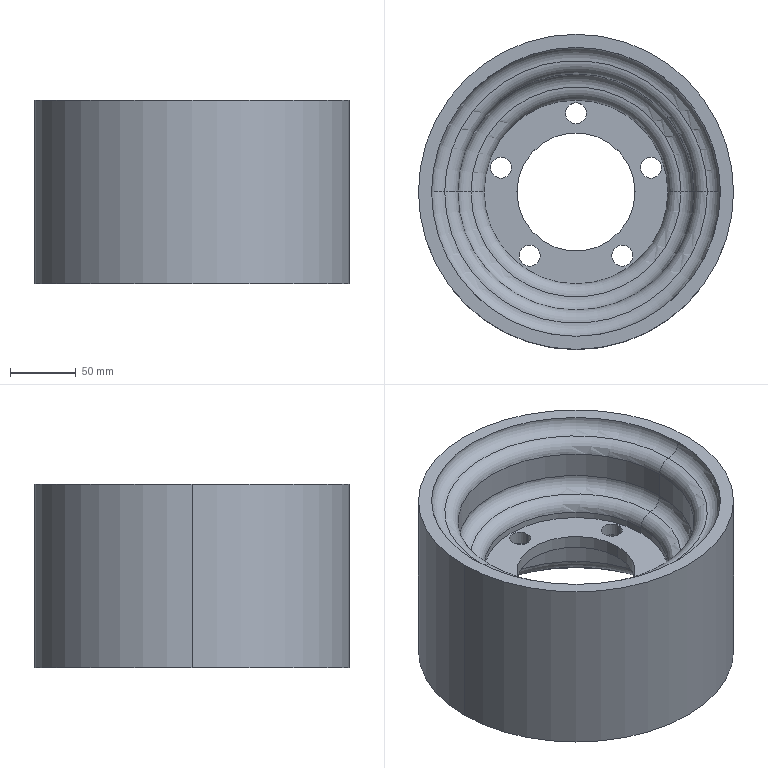Part | SolidWorks | features ICE 4, Extrusion 1, Fillet 1, MirrorPattern 1 | 1 solid | 42 faces | box 240 x 240 x 140 mm | volume 3010326 mm3 | cylinder 22 | torus 16 | plane 4 | commonest cylinder face diameters 16 x10 140 x4 180 x4 90 x2 240 x2
STEP:
#1=CARTESIAN_POINT('',(80.,0.,20.));
#2=VERTEX_POINT('',#1);
#3=CARTESIAN_POINT('',(-80.,0.,20.));
#4=VERTEX_POINT('',#3);
#5=CARTESIAN_POINT('',(0.,0.,20.));
#6=DIRECTION('',(0.,0.,-1.));
#7=DIRECTION('',(1.,0.,0.));
#8=AXIS2_PLACEMENT_3D('',#5,#6,#7);
#9=CIRCLE('',#8,80.);
#10=EDGE_CURVE('',#2,#4,#9,.T.);
#11=ORIENTED_EDGE('',*,*,#10,.T.);
#12=CARTESIAN_POINT('',(-90.,0.,30.));
#13=VERTEX_POINT('',#12);
#14=CARTESIAN_POINT('',(-80.,0.,30.));
#15=DIRECTION('',(0.,1.,0.));
#16=DIRECTION('',(-1.,0.,0.));
#17=AXIS2_PLACEMENT_3D('',#14,#15,#16);
#18=CIRCLE('',#17,10.);
#19=EDGE_CURVE('',#4,#13,#18,.T.);
#20=ORIENTED_EDGE('',*,*,#19,.T.);
#21=CARTESIAN_POINT('',(90.,0.,30.));
#22=VERTEX_POINT('',#21);
#23=CARTESIAN_POINT('',(0.,0.,30.));
#24=DIRECTION('',(0.,0.,-1.));
#25=DIRECTION('',(1.,0.,0.));
#26=AXIS2_PLACEMENT_3D('',#23,#24,#25);
#27=CIRCLE('',#26,90.);
#28=EDGE_CURVE('',#22,#13,#27,.T.);
#29=ORIENTED_EDGE('',*,*,#28,.F.);
#30=CARTESIAN_POINT('',(80.,0.,30.));
#31=DIRECTION('',(0.,-1.,0.));
#32=DIRECTION('',(0.,0.,-1.));
#33=AXIS2_PLACEMENT_3D('',#30,#31,#32);
#34=CIRCLE('',#33,10.);
#35=EDGE_CURVE('',#2,#22,#34,.T.);
#36=ORIENTED_EDGE('',*,*,#35,.F.);
#37=EDGE_LOOP('',(#11,#20,#29,#36));
#38=FACE_OUTER_BOUND('',#37,.T.);
#39=CARTESIAN_POINT('',(0.,0.,30.));
#40=DIRECTION('',(0.,0.,1.));
#41=DIRECTION('',(1.,0.,0.));
#42=AXIS2_PLACEMENT_3D('',#39,#40,#41);
#43=TOROIDAL_SURFACE('',#42,80.,10.);
#44=ADVANCED_FACE('',(#38),#43,.F.);
#45=CARTESIAN_POINT('',(0.,0.,20.));
#46=DIRECTION('',(0.,0.,-1.));
#47=DIRECTION('',(1.,0.,0.));
#48=AXIS2_PLACEMENT_3D('',#45,#46,#47);
#49=CIRCLE('',#48,80.);
#50=EDGE_CURVE('',#4,#2,#49,.T.);
#51=ORIENTED_EDGE('',*,*,#50,.F.);
#52=CARTESIAN_POINT('',(-70.,0.,10.));
#53=VERTEX_POINT('',#52);
#54=CARTESIAN_POINT('',(-80.,0.,10.));
#55=DIRECTION('',(0.,1.,0.));
#56=DIRECTION('',(-1.,0.,0.));
#57=AXIS2_PLACEMENT_3D('',#54,#55,#56);
#58=CIRCLE('',#57,10.);
#59=EDGE_CURVE('',#4,#53,#58,.T.);
#60=ORIENTED_EDGE('',*,*,#59,.T.);
#61=CARTESIAN_POINT('',(70.,0.,10.));
#62=VERTEX_POINT('',#61);
#63=CARTESIAN_POINT('',(0.,0.,10.));
#64=DIRECTION('',(0.,0.,1.));
#65=DIRECTION('',(1.,0.,0.));
#66=AXIS2_PLACEMENT_3D('',#63,#64,#65);
#67=CIRCLE('',#66,70.);
#68=EDGE_CURVE('',#62,#53,#67,.T.);
#69=ORIENTED_EDGE('',*,*,#68,.F.);
#70=CARTESIAN_POINT('',(80.,0.,10.));
#71=DIRECTION('',(0.,-1.,0.));
#72=DIRECTION('',(0.,0.,-1.));
#73=AXIS2_PLACEMENT_3D('',#70,#71,#72);
#74=CIRCLE('',#73,10.);
#75=EDGE_CURVE('',#2,#62,#74,.T.);
#76=ORIENTED_EDGE('',*,*,#75,.F.);
#77=EDGE_LOOP('',(#51,#60,#69,#76));
#78=FACE_OUTER_BOUND('',#77,.T.);
#79=CARTESIAN_POINT('',(0.,0.,10.));
#80=DIRECTION('',(0.,0.,1.));
#81=DIRECTION('',(1.,0.,0.));
#82=AXIS2_PLACEMENT_3D('',#79,#80,#81);
#83=TOROIDAL_SURFACE('',#82,80.,10.);
#84=ADVANCED_FACE('',(#78),#83,.T.);
#85=CARTESIAN_POINT('',(100.,0.,60.));
#86=VERTEX_POINT('',#85);
#87=CARTESIAN_POINT('',(-100.,0.,60.));
#88=VERTEX_POINT('',#87);
#89=CARTESIAN_POINT('',(0.,0.,60.));
#90=DIRECTION('',(0.,0.,-1.));
#91=DIRECTION('',(1.,0.,0.));
#92=AXIS2_PLACEMENT_3D('',#89,#90,#91);
#93=CIRCLE('',#92,100.);
#94=EDGE_CURVE('',#86,#88,#93,.T.);
#95=ORIENTED_EDGE('',*,*,#94,.T.);
#96=CARTESIAN_POINT('',(-110.,0.,70.));
#97=VERTEX_POINT('',#96);
#98=CARTESIAN_POINT('',(-100.,0.,70.));
#99=DIRECTION('',(0.,1.,0.));
#100=DIRECTION('',(-1.,0.,0.));
#101=AXIS2_PLACEMENT_3D('',#98,#99,#100);
#102=CIRCLE('',#101,10.);
#103=EDGE_CURVE('',#88,#97,#102,.T.);
#104=ORIENTED_EDGE('',*,*,#103,.T.);
#105=CARTESIAN_POINT('',(110.,0.,70.));
#106=VERTEX_POINT('',#105);
#107=CARTESIAN_POINT('',(0.,0.,70.));
#108=DIRECTION('',(0.,0.,1.));
#109=DIRECTION('',(1.,0.,0.));
#110=AXIS2_PLACEMENT_3D('',#107,#108,#109);
#111=CIRCLE('',#110,110.);
#112=EDGE_CURVE('',#97,#106,#111,.T.);
#113=ORIENTED_EDGE('',*,*,#112,.T.);
#114=CARTESIAN_POINT('',(100.,0.,70.));
#115=DIRECTION('',(0.,-1.,0.));
#116=DIRECTION('',(0.,0.,-1.));
#117=AXIS2_PLACEMENT_3D('',#114,#115,#116);
#118=CIRCLE('',#117,10.);
#119=EDGE_CURVE('',#86,#106,#118,.T.);
#120=ORIENTED_EDGE('',*,*,#119,.F.);
#121=EDGE_LOOP('',(#95,#104,#113,#120));
#122=FACE_OUTER_BOUND('',#121,.T.);
#123=CARTESIAN_POINT('',(0.,0.,70.));
#124=DIRECTION('',(0.,0.,1.));
#125=DIRECTION('',(1.,0.,0.));
#126=AXIS2_PLACEMENT_3D('',#123,#124,#125);
#127=TOROIDAL_SURFACE('',#126,100.,10.);
#128=ADVANCED_FACE('',(#122),#127,.F.);
#129=CARTESIAN_POINT('',(0.,0.,60.));
#130=DIRECTION('',(0.,0.,-1.));
#131=DIRECTION('',(1.,0.,0.));
#132=AXIS2_PLACEMENT_3D('',#129,#130,#131);
#133=CIRCLE('',#132,100.);
#134=EDGE_CURVE('',#88,#86,#133,.T.);
#135=ORIENTED_EDGE('',*,*,#134,.F.);
#136=CARTESIAN_POINT('',(-90.,0.,50.));
#137=VERTEX_POINT('',#136);
#138=CARTESIAN_POINT('',(-100.,0.,50.));
#139=DIRECTION('',(0.,1.,0.));
#140=DIRECTION('',(-1.,0.,0.));
#141=AXIS2_PLACEMENT_3D('',#138,#139,#140);
#142=CIRCLE('',#141,10.);
#143=EDGE_CURVE('',#88,#137,#142,.T.);
#144=ORIENTED_EDGE('',*,*,#143,.T.);
#145=CARTESIAN_POINT('',(90.,0.,50.));
#146=VERTEX_POINT('',#145);
#147=CARTESIAN_POINT('',(0.,0.,50.));
#148=DIRECTION('',(0.,0.,1.));
#149=DIRECTION('',(1.,0.,0.));
#150=AXIS2_PLACEMENT_3D('',#147,#148,#149);
#151=CIRCLE('',#150,90.);
#152=EDGE_CURVE('',#146,#137,#151,.T.);
#153=ORIENTED_EDGE('',*,*,#152,.F.);
#154=CARTESIAN_POINT('',(100.,0.,50.));
#155=DIRECTION('',(0.,-1.,0.));
#156=DIRECTION('',(0.,0.,-1.));
#157=AXIS2_PLACEMENT_3D('',#154,#155,#156);
#158=CIRCLE('',#157,10.);
#159=EDGE_CURVE('',#86,#146,#158,.T.);
#160=ORIENTED_EDGE('',*,*,#159,.F.);
#161=EDGE_LOOP('',(#135,#144,#153,#160));
#162=FACE_OUTER_BOUND('',#161,.T.);
#163=CARTESIAN_POINT('',(0.,0.,50.));
#164=DIRECTION('',(0.,0.,1.));
#165=DIRECTION('',(1.,0.,0.));
#166=AXIS2_PLACEMENT_3D('',#163,#164,#165);
#167=TOROIDAL_SURFACE('',#166,100.,10.);
#168=ADVANCED_FACE('',(#162),#167,.T.);
#169=CARTESIAN_POINT('',(-80.,0.,-20.));
#170=VERTEX_POINT('',#169);
#171=CARTESIAN_POINT('',(80.,0.,-20.));
#172=VERTEX_POINT('',#171);
#173=CARTESIAN_POINT('',(0.,0.,-20.));
#174=DIRECTION('',(0.,0.,1.));
#175=DIRECTION('',(-1.,0.,0.));
#176=AXIS2_PLACEMENT_3D('',#173,#174,#175);
#177=CIRCLE('',#176,80.);
#178=EDGE_CURVE('',#170,#172,#177,.T.);
#179=ORIENTED_EDGE('',*,*,#178,.T.);
#180=CARTESIAN_POINT('',(90.,0.,-30.));
#181=VERTEX_POINT('',#180);
#182=CARTESIAN_POINT('',(80.,0.,-30.));
#183=DIRECTION('',(0.,1.,0.));
#184=DIRECTION('',(-1.,0.,0.));
#185=AXIS2_PLACEMENT_3D('',#182,#183,#184);
#186=CIRCLE('',#185,10.);
#187=EDGE_CURVE('',#172,#181,#186,.T.);
#188=ORIENTED_EDGE('',*,*,#187,.T.);
#189=CARTESIAN_POINT('',(-90.,0.,-30.));
#190=VERTEX_POINT('',#189);
#191=CARTESIAN_POINT('',(0.,0.,-30.));
#192=DIRECTION('',(0.,0.,1.));
#193=DIRECTION('',(-1.,0.,0.));
#194=AXIS2_PLACEMENT_3D('',#191,#192,#193);
#195=CIRCLE('',#194,90.);
#196=EDGE_CURVE('',#190,#181,#195,.T.);
#197=ORIENTED_EDGE('',*,*,#196,.F.);
#198=CARTESIAN_POINT('',(-80.,0.,-30.));
#199=DIRECTION('',(0.,-1.,0.));
#200=DIRECTION('',(0.,0.,-1.));
#201=AXIS2_PLACEMENT_3D('',#198,#199,#200);
#202=CIRCLE('',#201,10.);
#203=EDGE_CURVE('',#170,#190,#202,.T.);
#204=ORIENTED_EDGE('',*,*,#203,.F.);
#205=EDGE_LOOP('',(#179,#188,#197,#204));
#206=FACE_OUTER_BOUND('',#205,.T.);
#207=CARTESIAN_POINT('',(0.,0.,-30.));
#208=DIRECTION('',(0.,0.,-1.));
#209=DIRECTION('',(-1.,0.,0.));
#210=AXIS2_PLACEMENT_3D('',#207,#208,#209);
#211=TOROIDAL_SURFACE('',#210,80.,10.);
#212=ADVANCED_FACE('',(#206),#211,.F.);
#213=CARTESIAN_POINT('',(0.,0.,-20.));
#214=DIRECTION('',(0.,0.,1.));
#215=DIRECTION('',(-1.,0.,0.));
#216=AXIS2_PLACEMENT_3D('',#213,#214,#215);
#217=CIRCLE('',#216,80.);
#218=EDGE_CURVE('',#172,#170,#217,.T.);
#219=ORIENTED_EDGE('',*,*,#218,.F.);
#220=CARTESIAN_POINT('',(70.,0.,-10.));
#221=VERTEX_POINT('',#220);
#222=CARTESIAN_POINT('',(80.,0.,-10.));
#223=DIRECTION('',(0.,1.,0.));
#224=DIRECTION('',(-1.,0.,0.));
#225=AXIS2_PLACEMENT_3D('',#222,#223,#224);
#226=CIRCLE('',#225,10.);
#227=EDGE_CURVE('',#172,#221,#226,.T.);
#228=ORIENTED_EDGE('',*,*,#227,.T.);
#229=CARTESIAN_POINT('',(-70.,0.,-10.));
#230=VERTEX_POINT('',#229);
#231=CARTESIAN_POINT('',(0.,0.,-10.));
#232=DIRECTION('',(0.,0.,-1.));
#233=DIRECTION('',(-1.,0.,0.));
#234=AXIS2_PLACEMENT_3D('',#231,#232,#233);
#235=CIRCLE('',#234,70.);
#236=EDGE_CURVE('',#230,#221,#235,.T.);
#237=ORIENTED_EDGE('',*,*,#236,.F.);
#238=CARTESIAN_POINT('',(-80.,0.,-10.));
#239=DIRECTION('',(0.,-1.,0.));
#240=DIRECTION('',(0.,0.,-1.));
#241=AXIS2_PLACEMENT_3D('',#238,#239,#240);
#242=CIRCLE('',#241,10.);
#243=EDGE_CURVE('',#170,#230,#242,.T.);
#244=ORIENTED_EDGE('',*,*,#243,.F.);
#245=EDGE_LOOP('',(#219,#228,#237,#244));
#246=FACE_OUTER_BOUND('',#245,.T.);
#247=CARTESIAN_POINT('',(0.,0.,-10.));
#248=DIRECTION('',(0.,0.,-1.));
#249=DIRECTION('',(-1.,0.,0.));
#250=AXIS2_PLACEMENT_3D('',#247,#248,#249);
#251=TOROIDAL_SURFACE('',#250,80.,10.);
#252=ADVANCED_FACE('',(#246),#251,.T.);
#253=CARTESIAN_POINT('',(-100.,0.,-60.));
#254=VERTEX_POINT('',#253);
#255=CARTESIAN_POINT('',(100.,0.,-60.));
#256=VERTEX_POINT('',#255);
#257=CARTESIAN_POINT('',(0.,0.,-60.));
#258=DIRECTION('',(0.,0.,1.));
#259=DIRECTION('',(-1.,0.,0.));
#260=AXIS2_PLACEMENT_3D('',#257,#258,#259);
#261=CIRCLE('',#260,100.);
#262=EDGE_CURVE('',#254,#256,#261,.T.);
#263=ORIENTED_EDGE('',*,*,#262,.T.);
#264=CARTESIAN_POINT('',(110.,0.,-70.));
#265=VERTEX_POINT('',#264);
#266=CARTESIAN_POINT('',(100.,0.,-70.));
#267=DIRECTION('',(0.,1.,0.));
#268=DIRECTION('',(-1.,0.,0.));
#269=AXIS2_PLACEMENT_3D('',#266,#267,#268);
#270=CIRCLE('',#269,10.);
#271=EDGE_CURVE('',#256,#265,#270,.T.);
#272=ORIENTED_EDGE('',*,*,#271,.T.);
#273=CARTESIAN_POINT('',(-110.,0.,-70.));
#274=VERTEX_POINT('',#273);
#275=CARTESIAN_POINT('',(0.,0.,-70.));
#276=DIRECTION('',(0.,0.,1.));
#277=DIRECTION('',(1.,0.,0.));
#278=AXIS2_PLACEMENT_3D('',#275,#276,#277);
#279=CIRCLE('',#278,110.);
#280=EDGE_CURVE('',#274,#265,#279,.T.);
#281=ORIENTED_EDGE('',*,*,#280,.F.);
#282=CARTESIAN_POINT('',(-100.,0.,-70.));
#283=DIRECTION('',(0.,-1.,0.));
#284=DIRECTION('',(0.,0.,-1.));
#285=AXIS2_PLACEMENT_3D('',#282,#283,#284);
#286=CIRCLE('',#285,10.);
#287=EDGE_CURVE('',#254,#274,#286,.T.);
#288=ORIENTED_EDGE('',*,*,#287,.F.);
#289=EDGE_LOOP('',(#263,#272,#281,#288));
#290=FACE_OUTER_BOUND('',#289,.T.);
#291=CARTESIAN_POINT('',(0.,0.,-70.));
#292=DIRECTION('',(0.,0.,-1.));
#293=DIRECTION('',(-1.,0.,0.));
#294=AXIS2_PLACEMENT_3D('',#291,#292,#293);
#295=TOROIDAL_SURFACE('',#294,100.,10.);
#296=ADVANCED_FACE('',(#290),#295,.F.);
#297=CARTESIAN_POINT('',(0.,0.,-60.));
#298=DIRECTION('',(0.,0.,1.));
#299=DIRECTION('',(-1.,0.,0.));
#300=AXIS2_PLACEMENT_3D('',#297,#298,#299);
#301=CIRCLE('',#300,100.);
#302=EDGE_CURVE('',#256,#254,#301,.T.);
#303=ORIENTED_EDGE('',*,*,#302,.F.);
#304=CARTESIAN_POINT('',(90.,0.,-50.));
#305=VERTEX_POINT('',#304);
#306=CARTESIAN_POINT('',(100.,0.,-50.));
#307=DIRECTION('',(0.,1.,0.));
#308=DIRECTION('',(-1.,0.,0.));
#309=AXIS2_PLACEMENT_3D('',#306,#307,#308);
#310=CIRCLE('',#309,10.);
#311=EDGE_CURVE('',#256,#305,#310,.T.);
#312=ORIENTED_EDGE('',*,*,#311,.T.);
#313=CARTESIAN_POINT('',(-90.,0.,-50.));
#314=VERTEX_POINT('',#313);
#315=CARTESIAN_POINT('',(0.,0.,-50.));
#316=DIRECTION('',(0.,0.,-1.));
#317=DIRECTION('',(-1.,0.,0.));
#318=AXIS2_PLACEMENT_3D('',#315,#316,#317);
#319=CIRCLE('',#318,90.);
#320=EDGE_CURVE('',#314,#305,#319,.T.);
#321=ORIENTED_EDGE('',*,*,#320,.F.);
#322=CARTESIAN_POINT('',(-100.,0.,-50.));
#323=DIRECTION('',(0.,-1.,0.));
#324=DIRECTION('',(0.,0.,-1.));
#325=AXIS2_PLACEMENT_3D('',#322,#323,#324);
#326=CIRCLE('',#325,10.);
#327=EDGE_CURVE('',#254,#314,#326,.T.);
#328=ORIENTED_EDGE('',*,*,#327,.F.);
#329=EDGE_LOOP('',(#303,#312,#321,#328));
#330=FACE_OUTER_BOUND('',#329,.T.);
#331=CARTESIAN_POINT('',(0.,0.,-50.));
#332=DIRECTION('',(0.,0.,-1.));
#333=DIRECTION('',(-1.,0.,0.));
#334=AXIS2_PLACEMENT_3D('',#331,#332,#333);
#335=TOROIDAL_SURFACE('',#334,100.,10.);
#336=ADVANCED_FACE('',(#330),#335,.T.);
#337=CARTESIAN_POINT('',(8.,60.,-5.));
#338=VERTEX_POINT('',#337);
#339=CARTESIAN_POINT('',(-8.,60.,-5.));
#340=VERTEX_POINT('',#339);
#341=CARTESIAN_POINT('',(0.,60.,-5.));
#342=DIRECTION('',(0.,0.,-1.));
#343=DIRECTION('',(-1.,0.,0.));
#344=AXIS2_PLACEMENT_3D('',#341,#342,#343);
#345=CIRCLE('',#344,8.);
#346=EDGE_CURVE('',#338,#340,#345,.T.);
#347=ORIENTED_EDGE('',*,*,#346,.T.);
#348=CARTESIAN_POINT('',(-8.,60.,5.));
#349=VERTEX_POINT('',#348);
#350=CARTESIAN_POINT('',(-8.,60.,-70.));
#351=DIRECTION('',(0.,0.,1.));
#352=VECTOR('',#351,1000.);
#353=LINE('',#350,#352);
#354=EDGE_CURVE('',#340,#349,#353,.T.);
#355=ORIENTED_EDGE('',*,*,#354,.T.);
#356=CARTESIAN_POINT('',(8.,60.,5.));
#357=VERTEX_POINT('',#356);
#358=CARTESIAN_POINT('',(0.,60.,5.));
#359=DIRECTION('',(0.,0.,1.));
#360=DIRECTION('',(1.,0.,0.));
#361=AXIS2_PLACEMENT_3D('',#358,#359,#360);
#362=CIRCLE('',#361,8.);
#363=EDGE_CURVE('',#349,#357,#362,.T.);
#364=ORIENTED_EDGE('',*,*,#363,.T.);
#365=CARTESIAN_POINT('',(8.,60.,-70.));
#366=DIRECTION('',(0.,0.,1.));
#367=VECTOR('',#366,1000.);
#368=LINE('',#365,#367);
#369=EDGE_CURVE('',#338,#357,#368,.T.);
#370=ORIENTED_EDGE('',*,*,#369,.F.);
#371=EDGE_LOOP('',(#347,#355,#364,#370));
#372=FACE_OUTER_BOUND('',#371,.T.);
#373=CARTESIAN_POINT('',(0.,60.,-70.));
#374=DIRECTION('',(0.,0.,1.));
#375=DIRECTION('',(1.,0.,0.));
#376=AXIS2_PLACEMENT_3D('',#373,#374,#375);
#377=CYLINDRICAL_SURFACE('',#376,8.);
#378=ADVANCED_FACE('',(#372),#377,.F.);
#379=CARTESIAN_POINT('',(65.063,18.541,-5.));
#380=VERTEX_POINT('',#379);
#381=CARTESIAN_POINT('',(49.063,18.541,-5.));
#382=VERTEX_POINT('',#381);
#383=CARTESIAN_POINT('',(57.063,18.541,-5.));
#384=DIRECTION('',(0.,0.,-1.));
#385=DIRECTION('',(-1.,0.,0.));
#386=AXIS2_PLACEMENT_3D('',#383,#384,#385);
#387=CIRCLE('',#386,8.);
#388=EDGE_CURVE('',#380,#382,#387,.T.);
#389=ORIENTED_EDGE('',*,*,#388,.T.);
#390=CARTESIAN_POINT('',(49.063,18.541,5.));
#391=VERTEX_POINT('',#390);
#392=CARTESIAN_POINT('',(49.063,18.541,-70.));
#393=DIRECTION('',(0.,0.,1.));
#394=VECTOR('',#393,1000.);
#395=LINE('',#392,#394);
#396=EDGE_CURVE('',#382,#391,#395,.T.);
#397=ORIENTED_EDGE('',*,*,#396,.T.);
#398=CARTESIAN_POINT('',(65.063,18.541,5.));
#399=VERTEX_POINT('',#398);
#400=CARTESIAN_POINT('',(57.063,18.541,5.));
#401=DIRECTION('',(0.,0.,1.));
#402=DIRECTION('',(1.,0.,0.));
#403=AXIS2_PLACEMENT_3D('',#400,#401,#402);
#404=CIRCLE('',#403,8.);
#405=EDGE_CURVE('',#391,#399,#404,.T.);
#406=ORIENTED_EDGE('',*,*,#405,.T.);
#407=CARTESIAN_POINT('',(65.063,18.541,-70.));
#408=DIRECTION('',(0.,0.,1.));
#409=VECTOR('',#408,1000.);
#410=LINE('',#407,#409);
#411=EDGE_CURVE('',#380,#399,#410,.T.);
#412=ORIENTED_EDGE('',*,*,#411,.F.);
#413=EDGE_LOOP('',(#389,#397,#406,#412));
#414=FACE_OUTER_BOUND('',#413,.T.);
#415=CARTESIAN_POINT('',(57.063,18.541,-70.));
#416=DIRECTION('',(0.,0.,1.));
#417=DIRECTION('',(1.,0.,0.));
#418=AXIS2_PLACEMENT_3D('',#415,#416,#417);
#419=CYLINDRICAL_SURFACE('',#418,8.);
#420=ADVANCED_FACE('',(#414),#419,.F.);
#421=CARTESIAN_POINT('',(43.267,-48.541,-5.));
#422=VERTEX_POINT('',#421);
#423=CARTESIAN_POINT('',(27.267,-48.541,-5.));
#424=VERTEX_POINT('',#423);
#425=CARTESIAN_POINT('',(35.267,-48.541,-5.));
#426=DIRECTION('',(0.,0.,-1.));
#427=DIRECTION('',(-1.,0.,0.));
#428=AXIS2_PLACEMENT_3D('',#425,#426,#427);
#429=CIRCLE('',#428,8.);
#430=EDGE_CURVE('',#422,#424,#429,.T.);
#431=ORIENTED_EDGE('',*,*,#430,.T.);
#432=CARTESIAN_POINT('',(27.267,-48.541,5.));
#433=VERTEX_POINT('',#432);
#434=CARTESIAN_POINT('',(27.267,-48.541,-70.));
#435=DIRECTION('',(0.,0.,1.));
#436=VECTOR('',#435,1000.);
#437=LINE('',#434,#436);
#438=EDGE_CURVE('',#424,#433,#437,.T.);
#439=ORIENTED_EDGE('',*,*,#438,.T.);
#440=CARTESIAN_POINT('',(43.267,-48.541,5.));
#441=VERTEX_POINT('',#440);
#442=CARTESIAN_POINT('',(35.267,-48.541,5.));
#443=DIRECTION('',(0.,0.,1.));
#444=DIRECTION('',(1.,0.,0.));
#445=AXIS2_PLACEMENT_3D('',#442,#443,#444);
#446=CIRCLE('',#445,8.);
#447=EDGE_CURVE('',#433,#441,#446,.T.);
#448=ORIENTED_EDGE('',*,*,#447,.T.);
#449=CARTESIAN_POINT('',(43.267,-48.541,-70.));
#450=DIRECTION('',(0.,0.,1.));
#451=VECTOR('',#450,1000.);
#452=LINE('',#449,#451);
#453=EDGE_CURVE('',#422,#441,#452,.T.);
#454=ORIENTED_EDGE('',*,*,#453,.F.);
#455=EDGE_LOOP('',(#431,#439,#448,#454));
#456=FACE_OUTER_BOUND('',#455,.T.);
#457=CARTESIAN_POINT('',(35.267,-48.541,-70.));
#458=DIRECTION('',(0.,0.,1.));
#459=DIRECTION('',(1.,0.,0.));
#460=AXIS2_PLACEMENT_3D('',#457,#458,#459);
#461=CYLINDRICAL_SURFACE('',#460,8.);
#462=ADVANCED_FACE('',(#456),#461,.F.);
#463=CARTESIAN_POINT('',(-27.267,-48.541,-5.));
#464=VERTEX_POINT('',#463);
#465=CARTESIAN_POINT('',(-43.267,-48.541,-5.));
#466=VERTEX_POINT('',#465);
#467=CARTESIAN_POINT('',(-35.267,-48.541,-5.));
#468=DIRECTION('',(0.,0.,-1.));
#469=DIRECTION('',(-1.,0.,0.));
#470=AXIS2_PLACEMENT_3D('',#467,#468,#469);
#471=CIRCLE('',#470,8.);
#472=EDGE_CURVE('',#464,#466,#471,.T.);
#473=ORIENTED_EDGE('',*,*,#472,.T.);
#474=CARTESIAN_POINT('',(-43.267,-48.541,5.));
#475=VERTEX_POINT('',#474);
#476=CARTESIAN_POINT('',(-43.267,-48.541,-70.));
#477=DIRECTION('',(0.,0.,1.));
#478=VECTOR('',#477,1000.);
#479=LINE('',#476,#478);
#480=EDGE_CURVE('',#466,#475,#479,.T.);
#481=ORIENTED_EDGE('',*,*,#480,.T.);
#482=CARTESIAN_POINT('',(-27.267,-48.541,5.));
#483=VERTEX_POINT('',#482);
#484=CARTESIAN_POINT('',(-35.267,-48.541,5.));
#485=DIRECTION('',(0.,0.,1.));
#486=DIRECTION('',(1.,0.,0.));
#487=AXIS2_PLACEMENT_3D('',#484,#485,#486);
#488=CIRCLE('',#487,8.);
#489=EDGE_CURVE('',#475,#483,#488,.T.);
#490=ORIENTED_EDGE('',*,*,#489,.T.);
#491=CARTESIAN_POINT('',(-27.267,-48.541,-70.));
#492=DIRECTION('',(0.,0.,1.));
#493=VECTOR('',#492,1000.);
#494=LINE('',#491,#493);
#495=EDGE_CURVE('',#464,#483,#494,.T.);
#496=ORIENTED_EDGE('',*,*,#495,.F.);
#497=EDGE_LOOP('',(#473,#481,#490,#496));
#498=FACE_OUTER_BOUND('',#497,.T.);
#499=CARTESIAN_POINT('',(-35.267,-48.541,-70.));
#500=DIRECTION('',(0.,0.,1.));
#501=DIRECTION('',(1.,0.,0.));
#502=AXIS2_PLACEMENT_3D('',#499,#500,#501);
#503=CYLINDRICAL_SURFACE('',#502,8.);
#504=ADVANCED_FACE('',(#498),#503,.F.);
#505=CARTESIAN_POINT('',(-49.063,18.541,-5.));
#506=VERTEX_POINT('',#505);
#507=CARTESIAN_POINT('',(-65.063,18.541,-5.));
#508=VERTEX_POINT('',#507);
#509=CARTESIAN_POINT('',(-57.063,18.541,-5.));
#510=DIRECTION('',(0.,0.,-1.));
#511=DIRECTION('',(-1.,0.,0.));
#512=AXIS2_PLACEMENT_3D('',#509,#510,#511);
#513=CIRCLE('',#512,8.);
#514=EDGE_CURVE('',#506,#508,#513,.T.);
#515=ORIENTED_EDGE('',*,*,#514,.T.);
#516=CARTESIAN_POINT('',(-65.063,18.541,5.));
#517=VERTEX_POINT('',#516);
#518=CARTESIAN_POINT('',(-65.063,18.541,-70.));
#519=DIRECTION('',(0.,0.,1.));
#520=VECTOR('',#519,1000.);
#521=LINE('',#518,#520);
#522=EDGE_CURVE('',#508,#517,#521,.T.);
#523=ORIENTED_EDGE('',*,*,#522,.T.);
#524=CARTESIAN_POINT('',(-49.063,18.541,5.));
#525=VERTEX_POINT('',#524);
#526=CARTESIAN_POINT('',(-57.063,18.541,5.));
#527=DIRECTION('',(0.,0.,1.));
#528=DIRECTION('',(1.,0.,0.));
#529=AXIS2_PLACEMENT_3D('',#526,#527,#528);
#530=CIRCLE('',#529,8.);
#531=EDGE_CURVE('',#517,#525,#530,.T.);
#532=ORIENTED_EDGE('',*,*,#531,.T.);
#533=CARTESIAN_POINT('',(-49.063,18.541,-70.));
#534=DIRECTION('',(0.,0.,1.));
#535=VECTOR('',#534,1000.);
#536=LINE('',#533,#535);
#537=EDGE_CURVE('',#506,#525,#536,.T.);
#538=ORIENTED_EDGE('',*,*,#537,.F.);
#539=EDGE_LOOP('',(#515,#523,#532,#538));
#540=FACE_OUTER_BOUND('',#539,.T.);
#541=CARTESIAN_POINT('',(-57.063,18.541,-70.));
#542=DIRECTION('',(0.,0.,1.));
#543=DIRECTION('',(1.,0.,0.));
#544=AXIS2_PLACEMENT_3D('',#541,#542,#543);
#545=CYLINDRICAL_SURFACE('',#544,8.);
#546=ADVANCED_FACE('',(#540),#545,.F.);
#547=CARTESIAN_POINT('',(-70.,0.,-5.));
#548=VERTEX_POINT('',#547);
#549=CARTESIAN_POINT('',(70.,0.,-5.));
#550=VERTEX_POINT('',#549);
#551=CARTESIAN_POINT('',(0.,0.,-5.));
#552=DIRECTION('',(0.,0.,1.));
#553=DIRECTION('',(1.,0.,0.));
#554=AXIS2_PLACEMENT_3D('',#551,#552,#553);
#555=CIRCLE('',#554,70.);
#556=EDGE_CURVE('',#548,#550,#555,.T.);
#557=ORIENTED_EDGE('',*,*,#556,.T.);
#558=CARTESIAN_POINT('',(70.,0.,-5.));
#559=DIRECTION('',(0.,0.,-1.));
#560=VECTOR('',#559,1000.);
#561=LINE('',#558,#560);
#562=EDGE_CURVE('',#550,#221,#561,.T.);
#563=ORIENTED_EDGE('',*,*,#562,.T.);
#564=CARTESIAN_POINT('',(0.,0.,-10.));
#565=DIRECTION('',(0.,0.,-1.));
#566=DIRECTION('',(-1.,0.,0.));
#567=AXIS2_PLACEMENT_3D('',#564,#565,#566);
#568=CIRCLE('',#567,70.);
#569=EDGE_CURVE('',#221,#230,#568,.T.);
#570=ORIENTED_EDGE('',*,*,#569,.T.);
#571=CARTESIAN_POINT('',(-70.,0.,-5.));
#572=DIRECTION('',(0.,0.,-1.));
#573=VECTOR('',#572,1000.);
#574=LINE('',#571,#573);
#575=EDGE_CURVE('',#548,#230,#574,.T.);
#576=ORIENTED_EDGE('',*,*,#575,.F.);
#577=EDGE_LOOP('',(#557,#563,#570,#576));
#578=FACE_OUTER_BOUND('',#577,.T.);
#579=CARTESIAN_POINT('',(0.,0.,-5.));
#580=DIRECTION('',(0.,0.,-1.));
#581=DIRECTION('',(-1.,0.,0.));
#582=AXIS2_PLACEMENT_3D('',#579,#580,#581);
#583=CYLINDRICAL_SURFACE('',#582,70.);
#584=ADVANCED_FACE('',(#578),#583,.F.);
#585=ORIENTED_EDGE('',*,*,#196,.T.);
#586=CARTESIAN_POINT('',(90.,0.,-20.));
#587=DIRECTION('',(0.,0.,-1.));
#588=VECTOR('',#587,1000.);
#589=LINE('',#586,#588);
#590=EDGE_CURVE('',#181,#305,#589,.T.);
#591=ORIENTED_EDGE('',*,*,#590,.T.);
#592=CARTESIAN_POINT('',(0.,0.,-50.));
#593=DIRECTION('',(0.,0.,-1.));
#594=DIRECTION('',(-1.,0.,0.));
#595=AXIS2_PLACEMENT_3D('',#592,#593,#594);
#596=CIRCLE('',#595,90.);
#597=EDGE_CURVE('',#305,#314,#596,.T.);
#598=ORIENTED_EDGE('',*,*,#597,.T.);
#599=CARTESIAN_POINT('',(-90.,0.,-20.));
#600=DIRECTION('',(0.,0.,-1.));
#601=VECTOR('',#600,1000.);
#602=LINE('',#599,#601);
#603=EDGE_CURVE('',#190,#314,#602,.T.);
#604=ORIENTED_EDGE('',*,*,#603,.F.);
#605=EDGE_LOOP('',(#585,#591,#598,#604));
#606=FACE_OUTER_BOUND('',#605,.T.);
#607=CARTESIAN_POINT('',(0.,0.,-20.));
#608=DIRECTION('',(0.,0.,-1.));
#609=DIRECTION('',(-1.,0.,0.));
#610=AXIS2_PLACEMENT_3D('',#607,#608,#609);
#611=CYLINDRICAL_SURFACE('',#610,90.);
#612=ADVANCED_FACE('',(#606),#611,.F.);
#613=CARTESIAN_POINT('',(-70.,0.,5.));
#614=VERTEX_POINT('',#613);
#615=CARTESIAN_POINT('',(70.,0.,5.));
#616=VERTEX_POINT('',#615);
#617=CARTESIAN_POINT('',(0.,0.,5.));
#618=DIRECTION('',(0.,0.,1.));
#619=DIRECTION('',(1.,0.,0.));
#620=AXIS2_PLACEMENT_3D('',#617,#618,#619);
#621=CIRCLE('',#620,70.);
#622=EDGE_CURVE('',#614,#616,#621,.T.);
#623=ORIENTED_EDGE('',*,*,#622,.F.);
#624=CARTESIAN_POINT('',(-70.,0.,5.));
#625=DIRECTION('',(0.,0.,1.));
#626=VECTOR('',#625,1000.);
#627=LINE('',#624,#626);
#628=EDGE_CURVE('',#614,#53,#627,.T.);
#629=ORIENTED_EDGE('',*,*,#628,.T.);
#630=CARTESIAN_POINT('',(0.,0.,10.));
#631=DIRECTION('',(0.,0.,1.));
#632=DIRECTION('',(1.,0.,0.));
#633=AXIS2_PLACEMENT_3D('',#630,#631,#632);
#634=CIRCLE('',#633,70.);
#635=EDGE_CURVE('',#53,#62,#634,.T.);
#636=ORIENTED_EDGE('',*,*,#635,.T.);
#637=CARTESIAN_POINT('',(70.,0.,5.));
#638=DIRECTION('',(0.,0.,1.));
#639=VECTOR('',#638,1000.);
#640=LINE('',#637,#639);
#641=EDGE_CURVE('',#616,#62,#640,.T.);
#642=ORIENTED_EDGE('',*,*,#641,.F.);
#643=EDGE_LOOP('',(#623,#629,#636,#642));
#644=FACE_OUTER_BOUND('',#643,.T.);
#645=CARTESIAN_POINT('',(0.,0.,5.));
#646=DIRECTION('',(0.,0.,1.));
#647=DIRECTION('',(1.,0.,0.));
#648=AXIS2_PLACEMENT_3D('',#645,#646,#647);
#649=CYLINDRICAL_SURFACE('',#648,70.);
#650=ADVANCED_FACE('',(#644),#649,.F.);
#651=ORIENTED_EDGE('',*,*,#28,.T.);
#652=CARTESIAN_POINT('',(-90.,0.,20.));
#653=DIRECTION('',(0.,0.,1.));
#654=VECTOR('',#653,1000.);
#655=LINE('',#652,#654);
#656=EDGE_CURVE('',#13,#137,#655,.T.);
#657=ORIENTED_EDGE('',*,*,#656,.T.);
#658=CARTESIAN_POINT('',(0.,0.,50.));
#659=DIRECTION('',(0.,0.,1.));
#660=DIRECTION('',(1.,0.,0.));
#661=AXIS2_PLACEMENT_3D('',#658,#659,#660);
#662=CIRCLE('',#661,90.);
#663=EDGE_CURVE('',#137,#146,#662,.T.);
#664=ORIENTED_EDGE('',*,*,#663,.T.);
#665=CARTESIAN_POINT('',(90.,0.,20.));
#666=DIRECTION('',(0.,0.,1.));
#667=VECTOR('',#666,1000.);
#668=LINE('',#665,#667);
#669=EDGE_CURVE('',#22,#146,#668,.T.);
#670=ORIENTED_EDGE('',*,*,#669,.F.);
#671=EDGE_LOOP('',(#651,#657,#664,#670));
#672=FACE_OUTER_BOUND('',#671,.T.);
#673=CARTESIAN_POINT('',(0.,0.,20.));
#674=DIRECTION('',(0.,0.,1.));
#675=DIRECTION('',(1.,0.,0.));
#676=AXIS2_PLACEMENT_3D('',#673,#674,#675);
#677=CYLINDRICAL_SURFACE('',#676,90.);
#678=ADVANCED_FACE('',(#672),#677,.F.);
#679=CARTESIAN_POINT('',(120.,0.,70.));
#680=VERTEX_POINT('',#679);
#681=CARTESIAN_POINT('',(-120.,0.,70.));
#682=VERTEX_POINT('',#681);
#683=CARTESIAN_POINT('',(0.,0.,70.));
#684=DIRECTION('',(0.,0.,1.));
#685=DIRECTION('',(1.,0.,0.));
#686=AXIS2_PLACEMENT_3D('',#683,#684,#685);
#687=CIRCLE('',#686,120.);
#688=EDGE_CURVE('',#680,#682,#687,.T.);
#689=ORIENTED_EDGE('',*,*,#688,.F.);
#690=CARTESIAN_POINT('',(120.,0.,-70.));
#691=VERTEX_POINT('',#690);
#692=CARTESIAN_POINT('',(120.,0.,70.));
#693=DIRECTION('',(0.,0.,-1.));
#694=VECTOR('',#693,1000.);
#695=LINE('',#692,#694);
#696=EDGE_CURVE('',#680,#691,#695,.T.);
#697=ORIENTED_EDGE('',*,*,#696,.T.);
#698=CARTESIAN_POINT('',(-120.,0.,-70.));
#699=VERTEX_POINT('',#698);
#700=CARTESIAN_POINT('',(0.,0.,-70.));
#701=DIRECTION('',(0.,0.,1.));
#702=DIRECTION('',(1.,0.,0.));
#703=AXIS2_PLACEMENT_3D('',#700,#701,#702);
#704=CIRCLE('',#703,120.);
#705=EDGE_CURVE('',#691,#699,#704,.T.);
#706=ORIENTED_EDGE('',*,*,#705,.T.);
#707=CARTESIAN_POINT('',(-120.,0.,70.));
#708=DIRECTION('',(0.,0.,-1.));
#709=VECTOR('',#708,1000.);
#710=LINE('',#707,#709);
#711=EDGE_CURVE('',#682,#699,#710,.T.);
#712=ORIENTED_EDGE('',*,*,#711,.F.);
#713=EDGE_LOOP('',(#689,#697,#706,#712));
#714=FACE_OUTER_BOUND('',#713,.T.);
#715=CARTESIAN_POINT('',(0.,0.,70.));
#716=DIRECTION('',(0.,0.,-1.));
#717=DIRECTION('',(-1.,0.,0.));
#718=AXIS2_PLACEMENT_3D('',#715,#716,#717);
#719=CYLINDRICAL_SURFACE('',#718,120.);
#720=ADVANCED_FACE('',(#714),#719,.T.);
#721=CARTESIAN_POINT('',(-45.,0.,5.));
#722=VERTEX_POINT('',#721);
#723=CARTESIAN_POINT('',(45.,0.,5.));
#724=VERTEX_POINT('',#723);
#725=CARTESIAN_POINT('',(0.,0.,5.));
#726=DIRECTION('',(0.,0.,1.));
#727=DIRECTION('',(1.,0.,0.));
#728=AXIS2_PLACEMENT_3D('',#725,#726,#727);
#729=CIRCLE('',#728,45.);
#730=EDGE_CURVE('',#722,#724,#729,.T.);
#731=ORIENTED_EDGE('',*,*,#730,.T.);
#732=CARTESIAN_POINT('',(45.,0.,-5.));
#733=VERTEX_POINT('',#732);
#734=CARTESIAN_POINT('',(45.,0.,70.));
#735=DIRECTION('',(0.,0.,-1.));
#736=VECTOR('',#735,1000.);
#737=LINE('',#734,#736);
#738=EDGE_CURVE('',#724,#733,#737,.T.);
#739=ORIENTED_EDGE('',*,*,#738,.T.);
#740=CARTESIAN_POINT('',(-45.,0.,-5.));
#741=VERTEX_POINT('',#740);
#742=CARTESIAN_POINT('',(0.,0.,-5.));
#743=DIRECTION('',(0.,0.,-1.));
#744=DIRECTION('',(-1.,0.,0.));
#745=AXIS2_PLACEMENT_3D('',#742,#743,#744);
#746=CIRCLE('',#745,45.);
#747=EDGE_CURVE('',#733,#741,#746,.T.);
#748=ORIENTED_EDGE('',*,*,#747,.T.);
#749=CARTESIAN_POINT('',(-45.,0.,70.));
#750=DIRECTION('',(0.,0.,-1.));
#751=VECTOR('',#750,1000.);
#752=LINE('',#749,#751);
#753=EDGE_CURVE('',#722,#741,#752,.T.);
#754=ORIENTED_EDGE('',*,*,#753,.F.);
#755=EDGE_LOOP('',(#731,#739,#748,#754));
#756=FACE_OUTER_BOUND('',#755,.T.);
#757=CARTESIAN_POINT('',(0.,0.,70.));
#758=DIRECTION('',(0.,0.,-1.));
#759=DIRECTION('',(-1.,0.,0.));
#760=AXIS2_PLACEMENT_3D('',#757,#758,#759);
#761=CYLINDRICAL_SURFACE('',#760,45.);
#762=ADVANCED_FACE('',(#756),#761,.F.);
#763=ORIENTED_EDGE('',*,*,#738,.F.);
#764=CARTESIAN_POINT('',(0.,0.,5.));
#765=DIRECTION('',(0.,0.,1.));
#766=DIRECTION('',(1.,0.,0.));
#767=AXIS2_PLACEMENT_3D('',#764,#765,#766);
#768=CIRCLE('',#767,45.);
#769=EDGE_CURVE('',#724,#722,#768,.T.);
#770=ORIENTED_EDGE('',*,*,#769,.T.);
#771=ORIENTED_EDGE('',*,*,#753,.T.);
#772=CARTESIAN_POINT('',(0.,0.,-5.));
#773=DIRECTION('',(0.,0.,-1.));
#774=DIRECTION('',(-1.,0.,0.));
#775=AXIS2_PLACEMENT_3D('',#772,#773,#774);
#776=CIRCLE('',#775,45.);
#777=EDGE_CURVE('',#741,#733,#776,.T.);
#778=ORIENTED_EDGE('',*,*,#777,.T.);
#779=EDGE_LOOP('',(#763,#770,#771,#778));
#780=FACE_OUTER_BOUND('',#779,.T.);
#781=CARTESIAN_POINT('',(0.,0.,70.));
#782=DIRECTION('',(0.,0.,-1.));
#783=DIRECTION('',(-1.,0.,0.));
#784=AXIS2_PLACEMENT_3D('',#781,#782,#783);
#785=CYLINDRICAL_SURFACE('',#784,45.);
#786=ADVANCED_FACE('',(#780),#785,.F.);
#787=CARTESIAN_POINT('',(0.,0.,70.));
#788=DIRECTION('',(0.,0.,1.));
#789=DIRECTION('',(1.,0.,0.));
#790=AXIS2_PLACEMENT_3D('',#787,#788,#789);
#791=CIRCLE('',#790,110.);
#792=EDGE_CURVE('',#106,#97,#791,.T.);
#793=ORIENTED_EDGE('',*,*,#792,.F.);
#794=ORIENTED_EDGE('',*,*,#112,.F.);
#795=EDGE_LOOP('',(#793,#794));
#796=FACE_BOUND('',#795,.T.);
#797=CARTESIAN_POINT('',(0.,0.,70.));
#798=DIRECTION('',(0.,0.,1.));
#799=DIRECTION('',(1.,0.,0.));
#800=AXIS2_PLACEMENT_3D('',#797,#798,#799);
#801=CIRCLE('',#800,120.);
#802=EDGE_CURVE('',#682,#680,#801,.T.);
#803=ORIENTED_EDGE('',*,*,#802,.T.);
#804=ORIENTED_EDGE('',*,*,#688,.T.);
#805=EDGE_LOOP('',(#803,#804));
#806=FACE_OUTER_BOUND('',#805,.T.);
#807=CARTESIAN_POINT('',(0.,0.,70.));
#808=DIRECTION('',(0.,0.,1.));
#809=DIRECTION('',(1.,0.,0.));
#810=AXIS2_PLACEMENT_3D('',#807,#808,#809);
#811=PLANE('',#810);
#812=ADVANCED_FACE('',(#796,#806),#811,.T.);
#813=ORIENTED_EDGE('',*,*,#280,.T.);
#814=CARTESIAN_POINT('',(0.,0.,-70.));
#815=DIRECTION('',(0.,0.,1.));
#816=DIRECTION('',(1.,0.,0.));
#817=AXIS2_PLACEMENT_3D('',#814,#815,#816);
#818=CIRCLE('',#817,110.);
#819=EDGE_CURVE('',#265,#274,#818,.T.);
#820=ORIENTED_EDGE('',*,*,#819,.T.);
#821=EDGE_LOOP('',(#813,#820));
#822=FACE_BOUND('',#821,.T.);
#823=CARTESIAN_POINT('',(0.,0.,-70.));
#824=DIRECTION('',(0.,0.,1.));
#825=DIRECTION('',(1.,0.,0.));
#826=AXIS2_PLACEMENT_3D('',#823,#824,#825);
#827=CIRCLE('',#826,120.);
#828=EDGE_CURVE('',#699,#691,#827,.T.);
#829=ORIENTED_EDGE('',*,*,#828,.F.);
#830=ORIENTED_EDGE('',*,*,#705,.F.);
#831=EDGE_LOOP('',(#829,#830));
#832=FACE_OUTER_BOUND('',#831,.T.);
#833=CARTESIAN_POINT('',(0.,0.,-70.));
#834=DIRECTION('',(0.,0.,1.));
#835=DIRECTION('',(1.,0.,0.));
#836=AXIS2_PLACEMENT_3D('',#833,#834,#835);
#837=PLANE('',#836);
#838=ADVANCED_FACE('',(#822,#832),#837,.F.);
#839=ORIENTED_EDGE('',*,*,#696,.F.);
#840=ORIENTED_EDGE('',*,*,#802,.F.);
#841=ORIENTED_EDGE('',*,*,#711,.T.);
#842=ORIENTED_EDGE('',*,*,#828,.T.);
#843=EDGE_LOOP('',(#839,#840,#841,#842));
#844=FACE_OUTER_BOUND('',#843,.T.);
#845=CARTESIAN_POINT('',(0.,0.,70.));
#846=DIRECTION('',(0.,0.,-1.));
#847=DIRECTION('',(-1.,0.,0.));
#848=AXIS2_PLACEMENT_3D('',#845,#846,#847);
#849=CYLINDRICAL_SURFACE('',#848,120.);
#850=ADVANCED_FACE('',(#844),#849,.T.);
#851=ORIENTED_EDGE('',*,*,#656,.F.);
#852=CARTESIAN_POINT('',(0.,0.,30.));
#853=DIRECTION('',(0.,0.,-1.));
#854=DIRECTION('',(1.,0.,0.));
#855=AXIS2_PLACEMENT_3D('',#852,#853,#854);
#856=CIRCLE('',#855,90.);
#857=EDGE_CURVE('',#13,#22,#856,.T.);
#858=ORIENTED_EDGE('',*,*,#857,.T.);
#859=ORIENTED_EDGE('',*,*,#669,.T.);
#860=ORIENTED_EDGE('',*,*,#152,.T.);
#861=EDGE_LOOP('',(#851,#858,#859,#860));
#862=FACE_OUTER_BOUND('',#861,.T.);
#863=CARTESIAN_POINT('',(0.,0.,20.));
#864=DIRECTION('',(0.,0.,1.));
#865=DIRECTION('',(1.,0.,0.));
#866=AXIS2_PLACEMENT_3D('',#863,#864,#865);
#867=CYLINDRICAL_SURFACE('',#866,90.);
#868=ADVANCED_FACE('',(#862),#867,.F.);
#869=ORIENTED_EDGE('',*,*,#628,.F.);
#870=CARTESIAN_POINT('',(0.,0.,5.));
#871=DIRECTION('',(0.,0.,1.));
#872=DIRECTION('',(1.,0.,0.));
#873=AXIS2_PLACEMENT_3D('',#870,#871,#872);
#874=CIRCLE('',#873,70.);
#875=EDGE_CURVE('',#616,#614,#874,.T.);
#876=ORIENTED_EDGE('',*,*,#875,.F.);
#877=ORIENTED_EDGE('',*,*,#641,.T.);
#878=ORIENTED_EDGE('',*,*,#68,.T.);
#879=EDGE_LOOP('',(#869,#876,#877,#878));
#880=FACE_OUTER_BOUND('',#879,.T.);
#881=CARTESIAN_POINT('',(0.,0.,5.));
#882=DIRECTION('',(0.,0.,1.));
#883=DIRECTION('',(1.,0.,0.));
#884=AXIS2_PLACEMENT_3D('',#881,#882,#883);
#885=CYLINDRICAL_SURFACE('',#884,70.);
#886=ADVANCED_FACE('',(#880),#885,.F.);
#887=CARTESIAN_POINT('',(0.,60.,5.));
#888=DIRECTION('',(0.,0.,1.));
#889=DIRECTION('',(1.,0.,0.));
#890=AXIS2_PLACEMENT_3D('',#887,#888,#889);
#891=CIRCLE('',#890,8.);
#892=EDGE_CURVE('',#357,#349,#891,.T.);
#893=ORIENTED_EDGE('',*,*,#892,.F.);
#894=ORIENTED_EDGE('',*,*,#363,.F.);
#895=EDGE_LOOP('',(#893,#894));
#896=FACE_BOUND('',#895,.T.);
#897=CARTESIAN_POINT('',(57.063,18.541,5.));
#898=DIRECTION('',(0.,0.,1.));
#899=DIRECTION('',(1.,0.,0.));
#900=AXIS2_PLACEMENT_3D('',#897,#898,#899);
#901=CIRCLE('',#900,8.);
#902=EDGE_CURVE('',#399,#391,#901,.T.);
#903=ORIENTED_EDGE('',*,*,#902,.F.);
#904=ORIENTED_EDGE('',*,*,#405,.F.);
#905=EDGE_LOOP('',(#903,#904));
#906=FACE_BOUND('',#905,.T.);
#907=CARTESIAN_POINT('',(35.267,-48.541,5.));
#908=DIRECTION('',(0.,0.,1.));
#909=DIRECTION('',(1.,0.,0.));
#910=AXIS2_PLACEMENT_3D('',#907,#908,#909);
#911=CIRCLE('',#910,8.);
#912=EDGE_CURVE('',#441,#433,#911,.T.);
#913=ORIENTED_EDGE('',*,*,#912,.F.);
#914=ORIENTED_EDGE('',*,*,#447,.F.);
#915=EDGE_LOOP('',(#913,#914));
#916=FACE_BOUND('',#915,.T.);
#917=CARTESIAN_POINT('',(-35.267,-48.541,5.));
#918=DIRECTION('',(0.,0.,1.));
#919=DIRECTION('',(1.,0.,0.));
#920=AXIS2_PLACEMENT_3D('',#917,#918,#919);
#921=CIRCLE('',#920,8.);
#922=EDGE_CURVE('',#483,#475,#921,.T.);
#923=ORIENTED_EDGE('',*,*,#922,.F.);
#924=ORIENTED_EDGE('',*,*,#489,.F.);
#925=EDGE_LOOP('',(#923,#924));
#926=FACE_BOUND('',#925,.T.);
#927=CARTESIAN_POINT('',(-57.063,18.541,5.));
#928=DIRECTION('',(0.,0.,1.));
#929=DIRECTION('',(1.,0.,0.));
#930=AXIS2_PLACEMENT_3D('',#927,#928,#929);
#931=CIRCLE('',#930,8.);
#932=EDGE_CURVE('',#525,#517,#931,.T.);
#933=ORIENTED_EDGE('',*,*,#932,.F.);
#934=ORIENTED_EDGE('',*,*,#531,.F.);
#935=EDGE_LOOP('',(#933,#934));
#936=FACE_BOUND('',#935,.T.);
#937=ORIENTED_EDGE('',*,*,#730,.F.);
#938=ORIENTED_EDGE('',*,*,#769,.F.);
#939=EDGE_LOOP('',(#937,#938));
#940=FACE_BOUND('',#939,.T.);
#941=ORIENTED_EDGE('',*,*,#875,.T.);
#942=ORIENTED_EDGE('',*,*,#622,.T.);
#943=EDGE_LOOP('',(#941,#942));
#944=FACE_OUTER_BOUND('',#943,.T.);
#945=CARTESIAN_POINT('',(0.,0.,5.));
#946=DIRECTION('',(0.,0.,1.));
#947=DIRECTION('',(1.,0.,0.));
#948=AXIS2_PLACEMENT_3D('',#945,#946,#947);
#949=PLANE('',#948);
#950=ADVANCED_FACE('',(#896,#906,#916,#926,#936,#940,#944),#949,.T.);
#951=ORIENTED_EDGE('',*,*,#590,.F.);
#952=CARTESIAN_POINT('',(0.,0.,-30.));
#953=DIRECTION('',(0.,0.,1.));
#954=DIRECTION('',(-1.,0.,0.));
#955=AXIS2_PLACEMENT_3D('',#952,#953,#954);
#956=CIRCLE('',#955,90.);
#957=EDGE_CURVE('',#181,#190,#956,.T.);
#958=ORIENTED_EDGE('',*,*,#957,.T.);
#959=ORIENTED_EDGE('',*,*,#603,.T.);
#960=ORIENTED_EDGE('',*,*,#320,.T.);
#961=EDGE_LOOP('',(#951,#958,#959,#960));
#962=FACE_OUTER_BOUND('',#961,.T.);
#963=CARTESIAN_POINT('',(0.,0.,-20.));
#964=DIRECTION('',(0.,0.,-1.));
#965=DIRECTION('',(-1.,0.,0.));
#966=AXIS2_PLACEMENT_3D('',#963,#964,#965);
#967=CYLINDRICAL_SURFACE('',#966,90.);
#968=ADVANCED_FACE('',(#962),#967,.F.);
#969=ORIENTED_EDGE('',*,*,#562,.F.);
#970=CARTESIAN_POINT('',(0.,0.,-5.));
#971=DIRECTION('',(0.,0.,1.));
#972=DIRECTION('',(1.,0.,0.));
#973=AXIS2_PLACEMENT_3D('',#970,#971,#972);
#974=CIRCLE('',#973,70.);
#975=EDGE_CURVE('',#550,#548,#974,.T.);
#976=ORIENTED_EDGE('',*,*,#975,.T.);
#977=ORIENTED_EDGE('',*,*,#575,.T.);
#978=ORIENTED_EDGE('',*,*,#236,.T.);
#979=EDGE_LOOP('',(#969,#976,#977,#978));
#980=FACE_OUTER_BOUND('',#979,.T.);
#981=CARTESIAN_POINT('',(0.,0.,-5.));
#982=DIRECTION('',(0.,0.,-1.));
#983=DIRECTION('',(-1.,0.,0.));
#984=AXIS2_PLACEMENT_3D('',#981,#982,#983);
#985=CYLINDRICAL_SURFACE('',#984,70.);
#986=ADVANCED_FACE('',(#980),#985,.F.);
#987=ORIENTED_EDGE('',*,*,#346,.F.);
#988=CARTESIAN_POINT('',(0.,60.,-5.));
#989=DIRECTION('',(0.,0.,-1.));
#990=DIRECTION('',(-1.,0.,0.));
#991=AXIS2_PLACEMENT_3D('',#988,#989,#990);
#992=CIRCLE('',#991,8.);
#993=EDGE_CURVE('',#340,#338,#992,.T.);
#994=ORIENTED_EDGE('',*,*,#993,.F.);
#995=EDGE_LOOP('',(#987,#994));
#996=FACE_BOUND('',#995,.T.);
#997=ORIENTED_EDGE('',*,*,#388,.F.);
#998=CARTESIAN_POINT('',(57.063,18.541,-5.));
#999=DIRECTION('',(0.,0.,-1.));
#1000=DIRECTION('',(-1.,0.,0.));
#1001=AXIS2_PLACEMENT_3D('',#998,#999,#1000);
#1002=CIRCLE('',#1001,8.);
#1003=EDGE_CURVE('',#382,#380,#1002,.T.);
#1004=ORIENTED_EDGE('',*,*,#1003,.F.);
#1005=EDGE_LOOP('',(#997,#1004));
#1006=FACE_BOUND('',#1005,.T.);
#1007=ORIENTED_EDGE('',*,*,#430,.F.);
#1008=CARTESIAN_POINT('',(35.267,-48.541,-5.));
#1009=DIRECTION('',(0.,0.,-1.));
#1010=DIRECTION('',(-1.,0.,0.));
#1011=AXIS2_PLACEMENT_3D('',#1008,#1009,#1010);
#1012=CIRCLE('',#1011,8.);
#1013=EDGE_CURVE('',#424,#422,#1012,.T.);
#1014=ORIENTED_EDGE('',*,*,#1013,.F.);
#1015=EDGE_LOOP('',(#1007,#1014));
#1016=FACE_BOUND('',#1015,.T.);
#1017=ORIENTED_EDGE('',*,*,#472,.F.);
#1018=CARTESIAN_POINT('',(-35.267,-48.541,-5.));
#1019=DIRECTION('',(0.,0.,-1.));
#1020=DIRECTION('',(-1.,0.,0.));
#1021=AXIS2_PLACEMENT_3D('',#1018,#1019,#1020);
#1022=CIRCLE('',#1021,8.);
#1023=EDGE_CURVE('',#466,#464,#1022,.T.);
#1024=ORIENTED_EDGE('',*,*,#1023,.F.);
#1025=EDGE_LOOP('',(#1017,#1024));
#1026=FACE_BOUND('',#1025,.T.);
#1027=ORIENTED_EDGE('',*,*,#514,.F.);
#1028=CARTESIAN_POINT('',(-57.063,18.541,-5.));
#1029=DIRECTION('',(0.,0.,-1.));
#1030=DIRECTION('',(-1.,0.,0.));
#1031=AXIS2_PLACEMENT_3D('',#1028,#1029,#1030);
#1032=CIRCLE('',#1031,8.);
#1033=EDGE_CURVE('',#508,#506,#1032,.T.);
#1034=ORIENTED_EDGE('',*,*,#1033,.F.);
#1035=EDGE_LOOP('',(#1027,#1034));
#1036=FACE_BOUND('',#1035,.T.);
#1037=ORIENTED_EDGE('',*,*,#777,.F.);
#1038=ORIENTED_EDGE('',*,*,#747,.F.);
#1039=EDGE_LOOP('',(#1037,#1038));
#1040=FACE_BOUND('',#1039,.T.);
#1041=ORIENTED_EDGE('',*,*,#556,.F.);
#1042=ORIENTED_EDGE('',*,*,#975,.F.);
#1043=EDGE_LOOP('',(#1041,#1042));
#1044=FACE_OUTER_BOUND('',#1043,.T.);
#1045=CARTESIAN_POINT('',(0.,0.,-5.));
#1046=DIRECTION('',(0.,0.,-1.));
#1047=DIRECTION('',(1.,0.,0.));
#1048=AXIS2_PLACEMENT_3D('',#1045,#1046,#1047);
#1049=PLANE('',#1048);
#1050=ADVANCED_FACE('',(#996,#1006,#1016,#1026,#1036,#1040,#1044),#1049,.T.);
#1051=ORIENTED_EDGE('',*,*,#522,.F.);
#1052=ORIENTED_EDGE('',*,*,#1033,.T.);
#1053=ORIENTED_EDGE('',*,*,#537,.T.);
#1054=ORIENTED_EDGE('',*,*,#932,.T.);
#1055=EDGE_LOOP('',(#1051,#1052,#1053,#1054));
#1056=FACE_OUTER_BOUND('',#1055,.T.);
#1057=CARTESIAN_POINT('',(-57.063,18.541,-70.));
#1058=DIRECTION('',(0.,0.,1.));
#1059=DIRECTION('',(1.,0.,0.));
#1060=AXIS2_PLACEMENT_3D('',#1057,#1058,#1059);
#1061=CYLINDRICAL_SURFACE('',#1060,8.);
#1062=ADVANCED_FACE('',(#1056),#1061,.F.);
#1063=ORIENTED_EDGE('',*,*,#480,.F.);
#1064=ORIENTED_EDGE('',*,*,#1023,.T.);
#1065=ORIENTED_EDGE('',*,*,#495,.T.);
#1066=ORIENTED_EDGE('',*,*,#922,.T.);
#1067=EDGE_LOOP('',(#1063,#1064,#1065,#1066));
#1068=FACE_OUTER_BOUND('',#1067,.T.);
#1069=CARTESIAN_POINT('',(-35.267,-48.541,-70.));
#1070=DIRECTION('',(0.,0.,1.));
#1071=DIRECTION('',(1.,0.,0.));
#1072=AXIS2_PLACEMENT_3D('',#1069,#1070,#1071);
#1073=CYLINDRICAL_SURFACE('',#1072,8.);
#1074=ADVANCED_FACE('',(#1068),#1073,.F.);
#1075=ORIENTED_EDGE('',*,*,#438,.F.);
#1076=ORIENTED_EDGE('',*,*,#1013,.T.);
#1077=ORIENTED_EDGE('',*,*,#453,.T.);
#1078=ORIENTED_EDGE('',*,*,#912,.T.);
#1079=EDGE_LOOP('',(#1075,#1076,#1077,#1078));
#1080=FACE_OUTER_BOUND('',#1079,.T.);
#1081=CARTESIAN_POINT('',(35.267,-48.541,-70.));
#1082=DIRECTION('',(0.,0.,1.));
#1083=DIRECTION('',(1.,0.,0.));
#1084=AXIS2_PLACEMENT_3D('',#1081,#1082,#1083);
#1085=CYLINDRICAL_SURFACE('',#1084,8.);
#1086=ADVANCED_FACE('',(#1080),#1085,.F.);
#1087=ORIENTED_EDGE('',*,*,#396,.F.);
#1088=ORIENTED_EDGE('',*,*,#1003,.T.);
#1089=ORIENTED_EDGE('',*,*,#411,.T.);
#1090=ORIENTED_EDGE('',*,*,#902,.T.);
#1091=EDGE_LOOP('',(#1087,#1088,#1089,#1090));
#1092=FACE_OUTER_BOUND('',#1091,.T.);
#1093=CARTESIAN_POINT('',(57.063,18.541,-70.));
#1094=DIRECTION('',(0.,0.,1.));
#1095=DIRECTION('',(1.,0.,0.));
#1096=AXIS2_PLACEMENT_3D('',#1093,#1094,#1095);
#1097=CYLINDRICAL_SURFACE('',#1096,8.);
#1098=ADVANCED_FACE('',(#1092),#1097,.F.);
#1099=ORIENTED_EDGE('',*,*,#354,.F.);
#1100=ORIENTED_EDGE('',*,*,#993,.T.);
#1101=ORIENTED_EDGE('',*,*,#369,.T.);
#1102=ORIENTED_EDGE('',*,*,#892,.T.);
#1103=EDGE_LOOP('',(#1099,#1100,#1101,#1102));
#1104=FACE_OUTER_BOUND('',#1103,.T.);
#1105=CARTESIAN_POINT('',(0.,60.,-70.));
#1106=DIRECTION('',(0.,0.,1.));
#1107=DIRECTION('',(1.,0.,0.));
#1108=AXIS2_PLACEMENT_3D('',#1105,#1106,#1107);
#1109=CYLINDRICAL_SURFACE('',#1108,8.);
#1110=ADVANCED_FACE('',(#1104),#1109,.F.);
#1111=ORIENTED_EDGE('',*,*,#311,.F.);
#1112=ORIENTED_EDGE('',*,*,#262,.F.);
#1113=ORIENTED_EDGE('',*,*,#327,.T.);
#1114=ORIENTED_EDGE('',*,*,#597,.F.);
#1115=EDGE_LOOP('',(#1111,#1112,#1113,#1114));
#1116=FACE_OUTER_BOUND('',#1115,.T.);
#1117=CARTESIAN_POINT('',(0.,0.,-50.));
#1118=DIRECTION('',(0.,0.,-1.));
#1119=DIRECTION('',(-1.,0.,0.));
#1120=AXIS2_PLACEMENT_3D('',#1117,#1118,#1119);
#1121=TOROIDAL_SURFACE('',#1120,100.,10.);
#1122=ADVANCED_FACE('',(#1116),#1121,.T.);
#1123=ORIENTED_EDGE('',*,*,#271,.F.);
#1124=ORIENTED_EDGE('',*,*,#302,.T.);
#1125=ORIENTED_EDGE('',*,*,#287,.T.);
#1126=ORIENTED_EDGE('',*,*,#819,.F.);
#1127=EDGE_LOOP('',(#1123,#1124,#1125,#1126));
#1128=FACE_OUTER_BOUND('',#1127,.T.);
#1129=CARTESIAN_POINT('',(0.,0.,-70.));
#1130=DIRECTION('',(0.,0.,-1.));
#1131=DIRECTION('',(-1.,0.,0.));
#1132=AXIS2_PLACEMENT_3D('',#1129,#1130,#1131);
#1133=TOROIDAL_SURFACE('',#1132,100.,10.);
#1134=ADVANCED_FACE('',(#1128),#1133,.F.);
#1135=ORIENTED_EDGE('',*,*,#227,.F.);
#1136=ORIENTED_EDGE('',*,*,#178,.F.);
#1137=ORIENTED_EDGE('',*,*,#243,.T.);
#1138=ORIENTED_EDGE('',*,*,#569,.F.);
#1139=EDGE_LOOP('',(#1135,#1136,#1137,#1138));
#1140=FACE_OUTER_BOUND('',#1139,.T.);
#1141=CARTESIAN_POINT('',(0.,0.,-10.));
#1142=DIRECTION('',(0.,0.,-1.));
#1143=DIRECTION('',(-1.,0.,0.));
#1144=AXIS2_PLACEMENT_3D('',#1141,#1142,#1143);
#1145=TOROIDAL_SURFACE('',#1144,80.,10.);
#1146=ADVANCED_FACE('',(#1140),#1145,.T.);
#1147=ORIENTED_EDGE('',*,*,#187,.F.);
#1148=ORIENTED_EDGE('',*,*,#218,.T.);
#1149=ORIENTED_EDGE('',*,*,#203,.T.);
#1150=ORIENTED_EDGE('',*,*,#957,.F.);
#1151=EDGE_LOOP('',(#1147,#1148,#1149,#1150));
#1152=FACE_OUTER_BOUND('',#1151,.T.);
#1153=CARTESIAN_POINT('',(0.,0.,-30.));
#1154=DIRECTION('',(0.,0.,-1.));
#1155=DIRECTION('',(-1.,0.,0.));
#1156=AXIS2_PLACEMENT_3D('',#1153,#1154,#1155);
#1157=TOROIDAL_SURFACE('',#1156,80.,10.);
#1158=ADVANCED_FACE('',(#1152),#1157,.F.);
#1159=ORIENTED_EDGE('',*,*,#143,.F.);
#1160=ORIENTED_EDGE('',*,*,#94,.F.);
#1161=ORIENTED_EDGE('',*,*,#159,.T.);
#1162=ORIENTED_EDGE('',*,*,#663,.F.);
#1163=EDGE_LOOP('',(#1159,#1160,#1161,#1162));
#1164=FACE_OUTER_BOUND('',#1163,.T.);
#1165=CARTESIAN_POINT('',(0.,0.,50.));
#1166=DIRECTION('',(0.,0.,1.));
#1167=DIRECTION('',(1.,0.,0.));
#1168=AXIS2_PLACEMENT_3D('',#1165,#1166,#1167);
#1169=TOROIDAL_SURFACE('',#1168,100.,10.);
#1170=ADVANCED_FACE('',(#1164),#1169,.T.);
#1171=ORIENTED_EDGE('',*,*,#103,.F.);
#1172=ORIENTED_EDGE('',*,*,#134,.T.);
#1173=ORIENTED_EDGE('',*,*,#119,.T.);
#1174=ORIENTED_EDGE('',*,*,#792,.T.);
#1175=EDGE_LOOP('',(#1171,#1172,#1173,#1174));
#1176=FACE_OUTER_BOUND('',#1175,.T.);
#1177=CARTESIAN_POINT('',(0.,0.,70.));
#1178=DIRECTION('',(0.,0.,1.));
#1179=DIRECTION('',(1.,0.,0.));
#1180=AXIS2_PLACEMENT_3D('',#1177,#1178,#1179);
#1181=TOROIDAL_SURFACE('',#1180,100.,10.);
#1182=ADVANCED_FACE('',(#1176),#1181,.F.);
#1183=ORIENTED_EDGE('',*,*,#59,.F.);
#1184=ORIENTED_EDGE('',*,*,#10,.F.);
#1185=ORIENTED_EDGE('',*,*,#75,.T.);
#1186=ORIENTED_EDGE('',*,*,#635,.F.);
#1187=EDGE_LOOP('',(#1183,#1184,#1185,#1186));
#1188=FACE_OUTER_BOUND('',#1187,.T.);
#1189=CARTESIAN_POINT('',(0.,0.,10.));
#1190=DIRECTION('',(0.,0.,1.));
#1191=DIRECTION('',(1.,0.,0.));
#1192=AXIS2_PLACEMENT_3D('',#1189,#1190,#1191);
#1193=TOROIDAL_SURFACE('',#1192,80.,10.);
#1194=ADVANCED_FACE('',(#1188),#1193,.T.);
#1195=ORIENTED_EDGE('',*,*,#19,.F.);
#1196=ORIENTED_EDGE('',*,*,#50,.T.);
#1197=ORIENTED_EDGE('',*,*,#35,.T.);
#1198=ORIENTED_EDGE('',*,*,#857,.F.);
#1199=EDGE_LOOP('',(#1195,#1196,#1197,#1198));
#1200=FACE_OUTER_BOUND('',#1199,.T.);
#1201=CARTESIAN_POINT('',(0.,0.,30.));
#1202=DIRECTION('',(0.,0.,1.));
#1203=DIRECTION('',(1.,0.,0.));
#1204=AXIS2_PLACEMENT_3D('',#1201,#1202,#1203);
#1205=TOROIDAL_SURFACE('',#1204,80.,10.);
#1206=ADVANCED_FACE('',(#1200),#1205,.F.);
#1207=CLOSED_SHELL('',(#44,#84,#128,#168,#212,#252,#296,#336,#378,#420,#462,#504,#546,#584,#612,#650,#678,#720,#762,#786,#812,#838,#850,#868,#886,#950,#968,#986,#1050,#1062,#1074,#1086,#1098,#1110,#1122,#1134,#1146,#1158,#1170,#1182,#1194,#1206));
#1208=MANIFOLD_SOLID_BREP('',#1207);
#1209=CARTESIAN_POINT('',(0.,0.,0.));
#1210=DIRECTION('',(0.,0.,1.));
#1211=DIRECTION('',(1.,0.,0.));
#1212=AXIS2_PLACEMENT_3D('',#1209,#1210,#1211);
#1213=(LENGTH_UNIT()NAMED_UNIT(*)SI_UNIT(.MILLI.,.METRE.));
#1214=UNCERTAINTY_MEASURE_WITH_UNIT(LENGTH_MEASURE(0.00001),#1213,'','');
#1215=(NAMED_UNIT(*)PLANE_ANGLE_UNIT()SI_UNIT($,.RADIAN.));
#1216=(NAMED_UNIT(*)SI_UNIT($,.STERADIAN.)SOLID_ANGLE_UNIT());
#1217=(GEOMETRIC_REPRESENTATION_CONTEXT(3)GLOBAL_UNCERTAINTY_ASSIGNED_CONTEXT((#1214))GLOBAL_UNIT_ASSIGNED_CONTEXT((#1213,#1215,#1216))REPRESENTATION_CONTEXT('',''));
#1218=ADVANCED_BREP_SHAPE_REPRESENTATION('',(#1208,#1212),#1217);